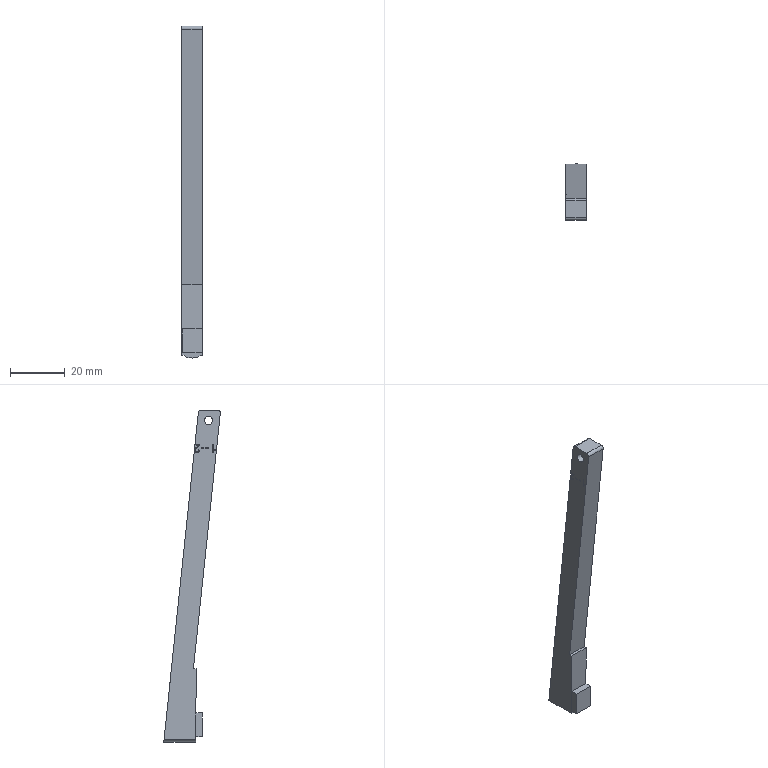Part | STEP file | solid 85 | 1 solid | 38 faces | box 7.5 x 20.679 x 121.269 mm | volume 7846 mm3 | plane 29 | other 5 | cylinder 4 | commonest cylinder face diameters 2 x2 3 x1 12.562 x1